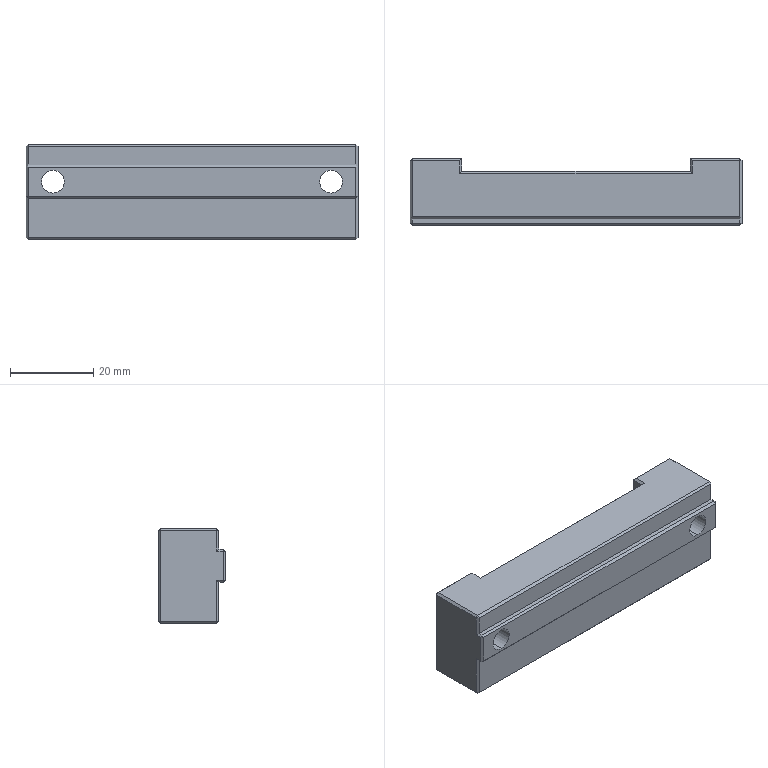Part | STEP file | PN_0006 fixture positioning -V-shape edge 2-2_Default | 1 solid | 82 faces | box 80 x 16 x 23 mm | volume 22056 mm3 | plane 58 | cylinder 16 | cone 8 | commonest cylinder face diameters 3.3 x8 5.5 x4 10 x4